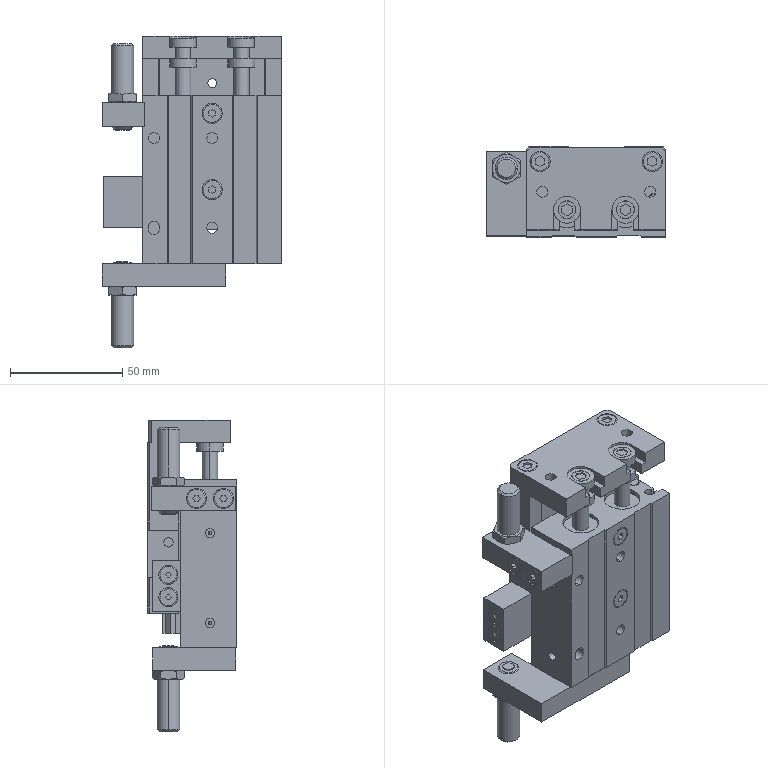Part | SolidWorks | features AEMSimFeature 1, Attribute 1 | 7 solids | 585 faces | box 80 x 40 x 138.911 mm | volume 215455 mm3 | plane 349 | cylinder 174 | cone 32 | spline 30 | commonest cylinder face diameters 4.134 x28 5 x23 9 x20 16 x16 4 x11 7 x10